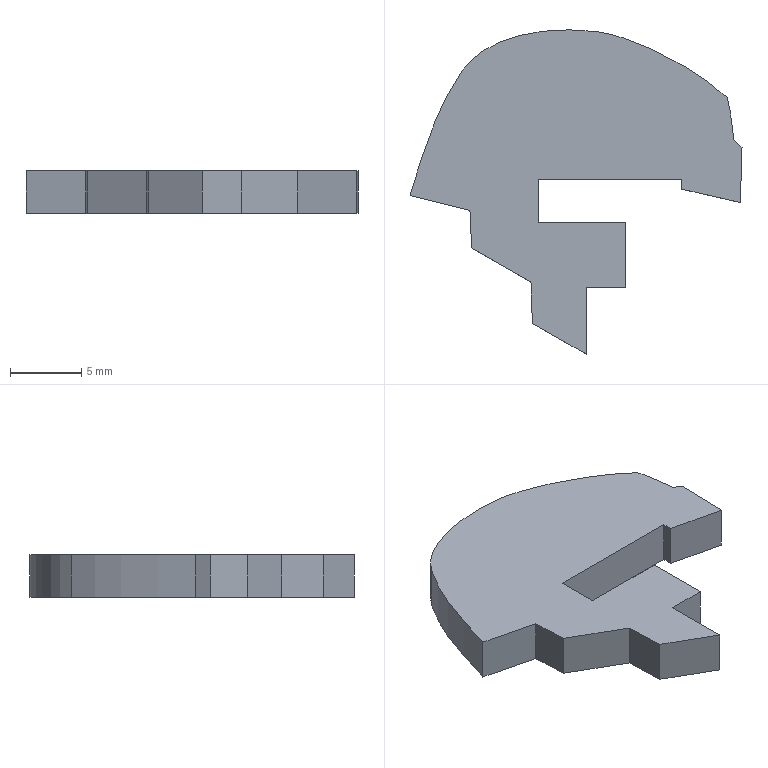Part | SolidWorks | features BaseBody 1 | 1 solid | 22 faces | box 23.312 x 22.774 x 3 mm | volume 818.077 mm3 | plane 18 | spline 4
STEP:
#1=CARTESIAN_POINT('',(21.406,16.89,-1.5));
#2=VERTEX_POINT('',#1);
#3=CARTESIAN_POINT('',(21.406,16.89,-1.5));
#4=VERTEX_POINT('',#3);
#5=CARTESIAN_POINT('',(21.406,16.89,-1.5));
#6=CARTESIAN_POINT('',(21.406,16.89,-1.5));
#7=CARTESIAN_POINT('',(21.406,16.89,-1.5));
#8=CARTESIAN_POINT('',(21.406,16.89,-1.5));
#9=B_SPLINE_CURVE_WITH_KNOTS('',3,(#5,#6,#7,#8),.UNSPECIFIED.,.F.,.F.,(4,4),(0.,0.000000108),.UNSPECIFIED.);
#10=EDGE_CURVE('',#2,#4,#9,.T.);
#11=ORIENTED_EDGE('',*,*,#10,.F.);
#12=CARTESIAN_POINT('',(25.034,25.614,-1.5));
#13=VERTEX_POINT('',#12);
#14=CARTESIAN_POINT('',(25.034,25.614,-1.5));
#15=CARTESIAN_POINT('',(23.262,23.049,-1.5));
#16=CARTESIAN_POINT('',(22.335,19.969,-1.5));
#17=CARTESIAN_POINT('',(21.406,16.89,-1.5));
#18=B_SPLINE_CURVE_WITH_KNOTS('',3,(#14,#15,#16,#17),.UNSPECIFIED.,.F.,.F.,(4,4),(0.000000108,0.03704),.UNSPECIFIED.);
#19=EDGE_CURVE('',#13,#2,#18,.T.);
#20=ORIENTED_EDGE('',*,*,#19,.F.);
#21=CARTESIAN_POINT('',(34.487,28.405,-1.5));
#22=VERTEX_POINT('',#21);
#23=CARTESIAN_POINT('',(34.487,28.405,-1.5));
#24=CARTESIAN_POINT('',(30.775,28.862,-1.5));
#25=CARTESIAN_POINT('',(26.734,28.074,-1.5));
#26=CARTESIAN_POINT('',(25.034,25.614,-1.5));
#27=B_SPLINE_CURVE_WITH_KNOTS('',3,(#23,#24,#25,#26),.UNSPECIFIED.,.F.,.F.,(4,4),(0.03704,0.07407),.UNSPECIFIED.);
#28=EDGE_CURVE('',#22,#13,#27,.T.);
#29=ORIENTED_EDGE('',*,*,#28,.F.);
#30=CARTESIAN_POINT('',(43.675,23.77,-1.5));
#31=VERTEX_POINT('',#30);
#32=CARTESIAN_POINT('',(43.675,23.77,-1.5));
#33=CARTESIAN_POINT('',(41.477,25.846,-1.5));
#34=CARTESIAN_POINT('',(37.107,28.083,-1.5));
#35=CARTESIAN_POINT('',(34.487,28.405,-1.5));
#36=B_SPLINE_CURVE_WITH_KNOTS('',3,(#32,#33,#34,#35),.UNSPECIFIED.,.F.,.F.,(4,4),(0.07407,0.1111),.UNSPECIFIED.);
#37=EDGE_CURVE('',#31,#22,#36,.T.);
#38=ORIENTED_EDGE('',*,*,#37,.F.);
#39=CARTESIAN_POINT('',(44.146,20.823,-1.5));
#40=VERTEX_POINT('',#39);
#41=CARTESIAN_POINT('',(44.146,20.823,-1.5));
#42=CARTESIAN_POINT('',(44.01,22.01,-1.5));
#43=CARTESIAN_POINT('',(43.871,23.199,-1.5));
#44=CARTESIAN_POINT('',(43.675,23.77,-1.5));
#45=B_SPLINE_CURVE_WITH_KNOTS('',3,(#41,#42,#43,#44),.UNSPECIFIED.,.F.,.F.,(4,4),(0.1111,0.1481),.UNSPECIFIED.);
#46=EDGE_CURVE('',#40,#31,#45,.T.);
#47=ORIENTED_EDGE('',*,*,#46,.F.);
#48=CARTESIAN_POINT('',(44.718,20.295,-1.5));
#49=VERTEX_POINT('',#48);
#50=CARTESIAN_POINT('',(44.718,20.295,-1.5));
#51=DIRECTION('',(-0.7346,0.6785,0.));
#52=VECTOR('',#51,1000.);
#53=LINE('',#50,#52);
#54=EDGE_CURVE('',#49,#40,#53,.T.);
#55=ORIENTED_EDGE('',*,*,#54,.F.);
#56=CARTESIAN_POINT('',(44.602,16.396,-1.5));
#57=VERTEX_POINT('',#56);
#58=CARTESIAN_POINT('',(44.602,16.396,-1.5));
#59=DIRECTION('',(0.02986,0.9996,0.));
#60=VECTOR('',#59,1000.);
#61=LINE('',#58,#60);
#62=EDGE_CURVE('',#57,#49,#61,.T.);
#63=ORIENTED_EDGE('',*,*,#62,.F.);
#64=CARTESIAN_POINT('',(40.499,17.339,-1.5));
#65=VERTEX_POINT('',#64);
#66=CARTESIAN_POINT('',(40.499,17.339,-1.5));
#67=DIRECTION('',(0.9746,-0.224,0.));
#68=VECTOR('',#67,1000.);
#69=LINE('',#66,#68);
#70=EDGE_CURVE('',#65,#57,#69,.T.);
#71=ORIENTED_EDGE('',*,*,#70,.F.);
#72=CARTESIAN_POINT('',(40.499,18.018,-1.5));
#73=VERTEX_POINT('',#72);
#74=CARTESIAN_POINT('',(40.499,18.018,-1.5));
#75=DIRECTION('',(0.,-1.,0.));
#76=VECTOR('',#75,1000.);
#77=LINE('',#74,#76);
#78=EDGE_CURVE('',#73,#65,#77,.T.);
#79=ORIENTED_EDGE('',*,*,#78,.F.);
#80=CARTESIAN_POINT('',(30.416,18.018,-1.5));
#81=VERTEX_POINT('',#80);
#82=CARTESIAN_POINT('',(30.416,18.018,-1.5));
#83=DIRECTION('',(1.,0.,0.));
#84=VECTOR('',#83,1000.);
#85=LINE('',#82,#84);
#86=EDGE_CURVE('',#81,#73,#85,.T.);
#87=ORIENTED_EDGE('',*,*,#86,.F.);
#88=CARTESIAN_POINT('',(30.416,15.018,-1.5));
#89=VERTEX_POINT('',#88);
#90=CARTESIAN_POINT('',(30.416,15.018,-1.5));
#91=DIRECTION('',(0.,1.,0.));
#92=VECTOR('',#91,1000.);
#93=LINE('',#90,#92);
#94=EDGE_CURVE('',#89,#81,#93,.T.);
#95=ORIENTED_EDGE('',*,*,#94,.F.);
#96=CARTESIAN_POINT('',(36.549,15.018,-1.5));
#97=VERTEX_POINT('',#96);
#98=CARTESIAN_POINT('',(36.549,15.018,-1.5));
#99=DIRECTION('',(-1.,0.,0.));
#100=VECTOR('',#99,1000.);
#101=LINE('',#98,#100);
#102=EDGE_CURVE('',#97,#89,#101,.T.);
#103=ORIENTED_EDGE('',*,*,#102,.F.);
#104=CARTESIAN_POINT('',(36.549,10.438,-1.5));
#105=VERTEX_POINT('',#104);
#106=CARTESIAN_POINT('',(36.549,10.438,-1.5));
#107=DIRECTION('',(0.,1.,0.));
#108=VECTOR('',#107,1000.);
#109=LINE('',#106,#108);
#110=EDGE_CURVE('',#105,#97,#109,.T.);
#111=ORIENTED_EDGE('',*,*,#110,.F.);
#112=CARTESIAN_POINT('',(33.779,10.438,-1.5));
#113=VERTEX_POINT('',#112);
#114=CARTESIAN_POINT('',(33.779,10.438,-1.5));
#115=DIRECTION('',(1.,0.,0.));
#116=VECTOR('',#115,1000.);
#117=LINE('',#114,#116);
#118=EDGE_CURVE('',#113,#105,#117,.T.);
#119=ORIENTED_EDGE('',*,*,#118,.F.);
#120=CARTESIAN_POINT('',(33.779,5.755,-1.5));
#121=VERTEX_POINT('',#120);
#122=CARTESIAN_POINT('',(33.779,5.755,-1.5));
#123=DIRECTION('',(0.,1.,0.));
#124=VECTOR('',#123,1000.);
#125=LINE('',#122,#124);
#126=EDGE_CURVE('',#121,#113,#125,.T.);
#127=ORIENTED_EDGE('',*,*,#126,.F.);
#128=CARTESIAN_POINT('',(29.997,7.91,-1.5));
#129=VERTEX_POINT('',#128);
#130=CARTESIAN_POINT('',(29.997,7.91,-1.5));
#131=DIRECTION('',(0.8688,-0.4952,0.));
#132=VECTOR('',#131,1000.);
#133=LINE('',#130,#132);
#134=EDGE_CURVE('',#129,#121,#133,.T.);
#135=ORIENTED_EDGE('',*,*,#134,.F.);
#136=CARTESIAN_POINT('',(29.9,10.832,-1.5));
#137=VERTEX_POINT('',#136);
#138=CARTESIAN_POINT('',(29.9,10.832,-1.5));
#139=DIRECTION('',(0.03337,-0.9994,0.));
#140=VECTOR('',#139,1000.);
#141=LINE('',#138,#140);
#142=EDGE_CURVE('',#137,#129,#141,.T.);
#143=ORIENTED_EDGE('',*,*,#142,.F.);
#144=CARTESIAN_POINT('',(25.734,13.212,-1.5));
#145=VERTEX_POINT('',#144);
#146=CARTESIAN_POINT('',(25.734,13.212,-1.5));
#147=DIRECTION('',(0.8682,-0.4962,0.));
#148=VECTOR('',#147,1000.);
#149=LINE('',#146,#148);
#150=EDGE_CURVE('',#145,#137,#149,.T.);
#151=ORIENTED_EDGE('',*,*,#150,.F.);
#152=CARTESIAN_POINT('',(25.615,15.852,-1.5));
#153=VERTEX_POINT('',#152);
#154=CARTESIAN_POINT('',(25.615,15.852,-1.5));
#155=DIRECTION('',(0.04529,-0.999,0.));
#156=VECTOR('',#155,1000.);
#157=LINE('',#154,#156);
#158=EDGE_CURVE('',#153,#145,#157,.T.);
#159=ORIENTED_EDGE('',*,*,#158,.F.);
#160=CARTESIAN_POINT('',(21.406,16.89,-1.5));
#161=DIRECTION('',(0.9709,-0.2396,0.));
#162=VECTOR('',#161,1000.);
#163=LINE('',#160,#162);
#164=EDGE_CURVE('',#4,#153,#163,.T.);
#165=ORIENTED_EDGE('',*,*,#164,.F.);
#166=EDGE_LOOP('',(#11,#20,#29,#38,#47,#55,#63,#71,#79,#87,#95,#103,#111,#119,#127,#135,#143,#151,#159,#165));
#167=FACE_OUTER_BOUND('',#166,.T.);
#168=CARTESIAN_POINT('',(22.904,21.445,-1.5));
#169=DIRECTION('',(0.,0.,-1.));
#170=DIRECTION('',(0.,-1.,0.));
#171=AXIS2_PLACEMENT_3D('',#168,#169,#170);
#172=PLANE('',#171);
#173=ADVANCED_FACE('',(#167),#172,.T.);
#174=CARTESIAN_POINT('',(21.406,16.89,1.5));
#175=VERTEX_POINT('',#174);
#176=CARTESIAN_POINT('',(21.406,16.89,1.5));
#177=VERTEX_POINT('',#176);
#178=CARTESIAN_POINT('',(21.406,16.89,1.5));
#179=CARTESIAN_POINT('',(21.406,16.89,1.5));
#180=CARTESIAN_POINT('',(21.406,16.89,1.5));
#181=CARTESIAN_POINT('',(21.406,16.89,1.5));
#182=B_SPLINE_CURVE_WITH_KNOTS('',3,(#178,#179,#180,#181),.UNSPECIFIED.,.F.,.F.,(4,4),(0.,0.000000108),.UNSPECIFIED.);
#183=EDGE_CURVE('',#175,#177,#182,.T.);
#184=ORIENTED_EDGE('',*,*,#183,.T.);
#185=CARTESIAN_POINT('',(25.615,15.852,1.5));
#186=VERTEX_POINT('',#185);
#187=CARTESIAN_POINT('',(21.406,16.89,1.5));
#188=DIRECTION('',(0.9709,-0.2396,0.));
#189=VECTOR('',#188,1000.);
#190=LINE('',#187,#189);
#191=EDGE_CURVE('',#177,#186,#190,.T.);
#192=ORIENTED_EDGE('',*,*,#191,.T.);
#193=CARTESIAN_POINT('',(25.734,13.212,1.5));
#194=VERTEX_POINT('',#193);
#195=CARTESIAN_POINT('',(25.615,15.852,1.5));
#196=DIRECTION('',(0.04529,-0.999,0.));
#197=VECTOR('',#196,1000.);
#198=LINE('',#195,#197);
#199=EDGE_CURVE('',#186,#194,#198,.T.);
#200=ORIENTED_EDGE('',*,*,#199,.T.);
#201=CARTESIAN_POINT('',(29.9,10.832,1.5));
#202=VERTEX_POINT('',#201);
#203=CARTESIAN_POINT('',(25.734,13.212,1.5));
#204=DIRECTION('',(0.8682,-0.4962,0.));
#205=VECTOR('',#204,1000.);
#206=LINE('',#203,#205);
#207=EDGE_CURVE('',#194,#202,#206,.T.);
#208=ORIENTED_EDGE('',*,*,#207,.T.);
#209=CARTESIAN_POINT('',(29.997,7.91,1.5));
#210=VERTEX_POINT('',#209);
#211=CARTESIAN_POINT('',(29.9,10.832,1.5));
#212=DIRECTION('',(0.03337,-0.9994,0.));
#213=VECTOR('',#212,1000.);
#214=LINE('',#211,#213);
#215=EDGE_CURVE('',#202,#210,#214,.T.);
#216=ORIENTED_EDGE('',*,*,#215,.T.);
#217=CARTESIAN_POINT('',(33.779,5.755,1.5));
#218=VERTEX_POINT('',#217);
#219=CARTESIAN_POINT('',(29.997,7.91,1.5));
#220=DIRECTION('',(0.8688,-0.4952,0.));
#221=VECTOR('',#220,1000.);
#222=LINE('',#219,#221);
#223=EDGE_CURVE('',#210,#218,#222,.T.);
#224=ORIENTED_EDGE('',*,*,#223,.T.);
#225=CARTESIAN_POINT('',(33.779,10.438,1.5));
#226=VERTEX_POINT('',#225);
#227=CARTESIAN_POINT('',(33.779,5.755,1.5));
#228=DIRECTION('',(0.,1.,0.));
#229=VECTOR('',#228,1000.);
#230=LINE('',#227,#229);
#231=EDGE_CURVE('',#218,#226,#230,.T.);
#232=ORIENTED_EDGE('',*,*,#231,.T.);
#233=CARTESIAN_POINT('',(36.549,10.438,1.5));
#234=VERTEX_POINT('',#233);
#235=CARTESIAN_POINT('',(33.779,10.438,1.5));
#236=DIRECTION('',(1.,0.,0.));
#237=VECTOR('',#236,1000.);
#238=LINE('',#235,#237);
#239=EDGE_CURVE('',#226,#234,#238,.T.);
#240=ORIENTED_EDGE('',*,*,#239,.T.);
#241=CARTESIAN_POINT('',(36.549,15.018,1.5));
#242=VERTEX_POINT('',#241);
#243=CARTESIAN_POINT('',(36.549,10.438,1.5));
#244=DIRECTION('',(0.,1.,0.));
#245=VECTOR('',#244,1000.);
#246=LINE('',#243,#245);
#247=EDGE_CURVE('',#234,#242,#246,.T.);
#248=ORIENTED_EDGE('',*,*,#247,.T.);
#249=CARTESIAN_POINT('',(30.416,15.018,1.5));
#250=VERTEX_POINT('',#249);
#251=CARTESIAN_POINT('',(36.549,15.018,1.5));
#252=DIRECTION('',(-1.,0.,0.));
#253=VECTOR('',#252,1000.);
#254=LINE('',#251,#253);
#255=EDGE_CURVE('',#242,#250,#254,.T.);
#256=ORIENTED_EDGE('',*,*,#255,.T.);
#257=CARTESIAN_POINT('',(30.416,18.018,1.5));
#258=VERTEX_POINT('',#257);
#259=CARTESIAN_POINT('',(30.416,15.018,1.5));
#260=DIRECTION('',(0.,1.,0.));
#261=VECTOR('',#260,1000.);
#262=LINE('',#259,#261);
#263=EDGE_CURVE('',#250,#258,#262,.T.);
#264=ORIENTED_EDGE('',*,*,#263,.T.);
#265=CARTESIAN_POINT('',(40.499,18.018,1.5));
#266=VERTEX_POINT('',#265);
#267=CARTESIAN_POINT('',(30.416,18.018,1.5));
#268=DIRECTION('',(1.,0.,0.));
#269=VECTOR('',#268,1000.);
#270=LINE('',#267,#269);
#271=EDGE_CURVE('',#258,#266,#270,.T.);
#272=ORIENTED_EDGE('',*,*,#271,.T.);
#273=CARTESIAN_POINT('',(40.499,17.339,1.5));
#274=VERTEX_POINT('',#273);
#275=CARTESIAN_POINT('',(40.499,18.018,1.5));
#276=DIRECTION('',(0.,-1.,0.));
#277=VECTOR('',#276,1000.);
#278=LINE('',#275,#277);
#279=EDGE_CURVE('',#266,#274,#278,.T.);
#280=ORIENTED_EDGE('',*,*,#279,.T.);
#281=CARTESIAN_POINT('',(44.602,16.396,1.5));
#282=VERTEX_POINT('',#281);
#283=CARTESIAN_POINT('',(40.499,17.339,1.5));
#284=DIRECTION('',(0.9746,-0.224,0.));
#285=VECTOR('',#284,1000.);
#286=LINE('',#283,#285);
#287=EDGE_CURVE('',#274,#282,#286,.T.);
#288=ORIENTED_EDGE('',*,*,#287,.T.);
#289=CARTESIAN_POINT('',(44.718,20.295,1.5));
#290=VERTEX_POINT('',#289);
#291=CARTESIAN_POINT('',(44.602,16.396,1.5));
#292=DIRECTION('',(0.02986,0.9996,0.));
#293=VECTOR('',#292,1000.);
#294=LINE('',#291,#293);
#295=EDGE_CURVE('',#282,#290,#294,.T.);
#296=ORIENTED_EDGE('',*,*,#295,.T.);
#297=CARTESIAN_POINT('',(44.146,20.823,1.5));
#298=VERTEX_POINT('',#297);
#299=CARTESIAN_POINT('',(44.718,20.295,1.5));
#300=DIRECTION('',(-0.7346,0.6785,0.));
#301=VECTOR('',#300,1000.);
#302=LINE('',#299,#301);
#303=EDGE_CURVE('',#290,#298,#302,.T.);
#304=ORIENTED_EDGE('',*,*,#303,.T.);
#305=CARTESIAN_POINT('',(43.675,23.77,1.5));
#306=VERTEX_POINT('',#305);
#307=CARTESIAN_POINT('',(44.146,20.823,1.5));
#308=CARTESIAN_POINT('',(44.01,22.01,1.5));
#309=CARTESIAN_POINT('',(43.871,23.199,1.5));
#310=CARTESIAN_POINT('',(43.675,23.77,1.5));
#311=B_SPLINE_CURVE_WITH_KNOTS('',3,(#307,#308,#309,#310),.UNSPECIFIED.,.F.,.F.,(4,4),(0.1111,0.1481),.UNSPECIFIED.);
#312=EDGE_CURVE('',#298,#306,#311,.T.);
#313=ORIENTED_EDGE('',*,*,#312,.T.);
#314=CARTESIAN_POINT('',(34.487,28.405,1.5));
#315=VERTEX_POINT('',#314);
#316=CARTESIAN_POINT('',(43.675,23.77,1.5));
#317=CARTESIAN_POINT('',(41.477,25.846,1.5));
#318=CARTESIAN_POINT('',(37.107,28.083,1.5));
#319=CARTESIAN_POINT('',(34.487,28.405,1.5));
#320=B_SPLINE_CURVE_WITH_KNOTS('',3,(#316,#317,#318,#319),.UNSPECIFIED.,.F.,.F.,(4,4),(0.07407,0.1111),.UNSPECIFIED.);
#321=EDGE_CURVE('',#306,#315,#320,.T.);
#322=ORIENTED_EDGE('',*,*,#321,.T.);
#323=CARTESIAN_POINT('',(25.034,25.614,1.5));
#324=VERTEX_POINT('',#323);
#325=CARTESIAN_POINT('',(34.487,28.405,1.5));
#326=CARTESIAN_POINT('',(30.775,28.862,1.5));
#327=CARTESIAN_POINT('',(26.734,28.074,1.5));
#328=CARTESIAN_POINT('',(25.034,25.614,1.5));
#329=B_SPLINE_CURVE_WITH_KNOTS('',3,(#325,#326,#327,#328),.UNSPECIFIED.,.F.,.F.,(4,4),(0.03704,0.07407),.UNSPECIFIED.);
#330=EDGE_CURVE('',#315,#324,#329,.T.);
#331=ORIENTED_EDGE('',*,*,#330,.T.);
#332=CARTESIAN_POINT('',(25.034,25.614,1.5));
#333=CARTESIAN_POINT('',(23.262,23.049,1.5));
#334=CARTESIAN_POINT('',(22.335,19.969,1.5));
#335=CARTESIAN_POINT('',(21.406,16.89,1.5));
#336=B_SPLINE_CURVE_WITH_KNOTS('',3,(#332,#333,#334,#335),.UNSPECIFIED.,.F.,.F.,(4,4),(0.000000108,0.03704),.UNSPECIFIED.);
#337=EDGE_CURVE('',#324,#175,#336,.T.);
#338=ORIENTED_EDGE('',*,*,#337,.T.);
#339=EDGE_LOOP('',(#184,#192,#200,#208,#216,#224,#232,#240,#248,#256,#264,#272,#280,#288,#296,#304,#313,#322,#331,#338));
#340=FACE_OUTER_BOUND('',#339,.T.);
#341=CARTESIAN_POINT('',(22.904,21.445,1.5));
#342=DIRECTION('',(0.,0.,-1.));
#343=DIRECTION('',(0.,-1.,0.));
#344=AXIS2_PLACEMENT_3D('',#341,#342,#343);
#345=PLANE('',#344);
#346=ADVANCED_FACE('',(#340),#345,.F.);
#347=ORIENTED_EDGE('',*,*,#19,.T.);
#348=CARTESIAN_POINT('',(21.406,16.89,1.5));
#349=DIRECTION('',(0.,0.,-1.));
#350=VECTOR('',#349,1000.);
#351=LINE('',#348,#350);
#352=EDGE_CURVE('',#175,#2,#351,.T.);
#353=ORIENTED_EDGE('',*,*,#352,.F.);
#354=ORIENTED_EDGE('',*,*,#337,.F.);
#355=CARTESIAN_POINT('',(25.034,25.614,1.5));
#356=DIRECTION('',(0.,0.,-1.));
#357=VECTOR('',#356,1000.);
#358=LINE('',#355,#357);
#359=EDGE_CURVE('',#324,#13,#358,.T.);
#360=ORIENTED_EDGE('',*,*,#359,.T.);
#361=EDGE_LOOP('',(#347,#353,#354,#360));
#362=FACE_OUTER_BOUND('',#361,.T.);
#363=CARTESIAN_POINT('',(25.034,25.614,1.5));
#364=CARTESIAN_POINT('',(25.034,25.614,-1.5));
#365=CARTESIAN_POINT('',(23.262,23.049,1.5));
#366=CARTESIAN_POINT('',(23.262,23.049,-1.5));
#367=CARTESIAN_POINT('',(22.335,19.969,1.5));
#368=CARTESIAN_POINT('',(22.335,19.969,-1.5));
#369=CARTESIAN_POINT('',(21.406,16.89,1.5));
#370=CARTESIAN_POINT('',(21.406,16.89,-1.5));
#371=B_SPLINE_SURFACE_WITH_KNOTS('',3,1,((#363,#364),(#365,#366),(#367,#368),(#369,#370)),.UNSPECIFIED.,.F.,.F.,.F.,(4,4),(2,2),(0.000000108,0.03704),(0.,1.),.UNSPECIFIED.);
#372=ADVANCED_FACE('',(#362),#371,.F.);
#373=ORIENTED_EDGE('',*,*,#28,.T.);
#374=ORIENTED_EDGE('',*,*,#359,.F.);
#375=ORIENTED_EDGE('',*,*,#330,.F.);
#376=CARTESIAN_POINT('',(34.487,28.405,1.5));
#377=DIRECTION('',(0.,0.,-1.));
#378=VECTOR('',#377,1000.);
#379=LINE('',#376,#378);
#380=EDGE_CURVE('',#315,#22,#379,.T.);
#381=ORIENTED_EDGE('',*,*,#380,.T.);
#382=EDGE_LOOP('',(#373,#374,#375,#381));
#383=FACE_OUTER_BOUND('',#382,.T.);
#384=CARTESIAN_POINT('',(34.487,28.405,1.5));
#385=CARTESIAN_POINT('',(34.487,28.405,-1.5));
#386=CARTESIAN_POINT('',(30.775,28.862,1.5));
#387=CARTESIAN_POINT('',(30.775,28.862,-1.5));
#388=CARTESIAN_POINT('',(26.734,28.074,1.5));
#389=CARTESIAN_POINT('',(26.734,28.074,-1.5));
#390=CARTESIAN_POINT('',(25.034,25.614,1.5));
#391=CARTESIAN_POINT('',(25.034,25.614,-1.5));
#392=B_SPLINE_SURFACE_WITH_KNOTS('',3,1,((#384,#385),(#386,#387),(#388,#389),(#390,#391)),.UNSPECIFIED.,.F.,.F.,.F.,(4,4),(2,2),(0.03704,0.07407),(0.,1.),.UNSPECIFIED.);
#393=ADVANCED_FACE('',(#383),#392,.F.);
#394=ORIENTED_EDGE('',*,*,#37,.T.);
#395=ORIENTED_EDGE('',*,*,#380,.F.);
#396=ORIENTED_EDGE('',*,*,#321,.F.);
#397=CARTESIAN_POINT('',(43.675,23.77,1.5));
#398=DIRECTION('',(0.,0.,-1.));
#399=VECTOR('',#398,1000.);
#400=LINE('',#397,#399);
#401=EDGE_CURVE('',#306,#31,#400,.T.);
#402=ORIENTED_EDGE('',*,*,#401,.T.);
#403=EDGE_LOOP('',(#394,#395,#396,#402));
#404=FACE_OUTER_BOUND('',#403,.T.);
#405=CARTESIAN_POINT('',(43.675,23.77,1.5));
#406=CARTESIAN_POINT('',(43.675,23.77,-1.5));
#407=CARTESIAN_POINT('',(41.477,25.846,1.5));
#408=CARTESIAN_POINT('',(41.477,25.846,-1.5));
#409=CARTESIAN_POINT('',(37.107,28.083,1.5));
#410=CARTESIAN_POINT('',(37.107,28.083,-1.5));
#411=CARTESIAN_POINT('',(34.487,28.405,1.5));
#412=CARTESIAN_POINT('',(34.487,28.405,-1.5));
#413=B_SPLINE_SURFACE_WITH_KNOTS('',3,1,((#405,#406),(#407,#408),(#409,#410),(#411,#412)),.UNSPECIFIED.,.F.,.F.,.F.,(4,4),(2,2),(0.07407,0.1111),(0.,1.),.UNSPECIFIED.);
#414=ADVANCED_FACE('',(#404),#413,.F.);
#415=ORIENTED_EDGE('',*,*,#46,.T.);
#416=ORIENTED_EDGE('',*,*,#401,.F.);
#417=ORIENTED_EDGE('',*,*,#312,.F.);
#418=CARTESIAN_POINT('',(44.146,20.823,1.5));
#419=DIRECTION('',(0.,0.,-1.));
#420=VECTOR('',#419,1000.);
#421=LINE('',#418,#420);
#422=EDGE_CURVE('',#298,#40,#421,.T.);
#423=ORIENTED_EDGE('',*,*,#422,.T.);
#424=EDGE_LOOP('',(#415,#416,#417,#423));
#425=FACE_OUTER_BOUND('',#424,.T.);
#426=CARTESIAN_POINT('',(44.146,20.823,1.5));
#427=CARTESIAN_POINT('',(44.146,20.823,-1.5));
#428=CARTESIAN_POINT('',(44.01,22.01,1.5));
#429=CARTESIAN_POINT('',(44.01,22.01,-1.5));
#430=CARTESIAN_POINT('',(43.871,23.199,1.5));
#431=CARTESIAN_POINT('',(43.871,23.199,-1.5));
#432=CARTESIAN_POINT('',(43.675,23.77,1.5));
#433=CARTESIAN_POINT('',(43.675,23.77,-1.5));
#434=B_SPLINE_SURFACE_WITH_KNOTS('',3,1,((#426,#427),(#428,#429),(#430,#431),(#432,#433)),.UNSPECIFIED.,.F.,.F.,.F.,(4,4),(2,2),(0.1111,0.1481),(0.,1.),.UNSPECIFIED.);
#435=ADVANCED_FACE('',(#425),#434,.F.);
#436=ORIENTED_EDGE('',*,*,#54,.T.);
#437=ORIENTED_EDGE('',*,*,#422,.F.);
#438=ORIENTED_EDGE('',*,*,#303,.F.);
#439=CARTESIAN_POINT('',(44.718,20.295,1.5));
#440=DIRECTION('',(0.,0.,-1.));
#441=VECTOR('',#440,1000.);
#442=LINE('',#439,#441);
#443=EDGE_CURVE('',#290,#49,#442,.T.);
#444=ORIENTED_EDGE('',*,*,#443,.T.);
#445=EDGE_LOOP('',(#436,#437,#438,#444));
#446=FACE_OUTER_BOUND('',#445,.T.);
#447=CARTESIAN_POINT('',(44.718,20.295,1.5));
#448=DIRECTION('',(-0.6785,-0.7346,0.));
#449=DIRECTION('',(-0.7346,0.6785,0.));
#450=AXIS2_PLACEMENT_3D('',#447,#448,#449);
#451=PLANE('',#450);
#452=ADVANCED_FACE('',(#446),#451,.F.);
#453=ORIENTED_EDGE('',*,*,#62,.T.);
#454=ORIENTED_EDGE('',*,*,#443,.F.);
#455=ORIENTED_EDGE('',*,*,#295,.F.);
#456=CARTESIAN_POINT('',(44.602,16.396,1.5));
#457=DIRECTION('',(0.,0.,-1.));
#458=VECTOR('',#457,1000.);
#459=LINE('',#456,#458);
#460=EDGE_CURVE('',#282,#57,#459,.T.);
#461=ORIENTED_EDGE('',*,*,#460,.T.);
#462=EDGE_LOOP('',(#453,#454,#455,#461));
#463=FACE_OUTER_BOUND('',#462,.T.);
#464=CARTESIAN_POINT('',(44.602,16.396,1.5));
#465=DIRECTION('',(-0.9996,0.02986,0.));
#466=DIRECTION('',(0.,0.,1.));
#467=AXIS2_PLACEMENT_3D('',#464,#465,#466);
#468=PLANE('',#467);
#469=ADVANCED_FACE('',(#463),#468,.F.);
#470=ORIENTED_EDGE('',*,*,#70,.T.);
#471=ORIENTED_EDGE('',*,*,#460,.F.);
#472=ORIENTED_EDGE('',*,*,#287,.F.);
#473=CARTESIAN_POINT('',(40.499,17.339,1.5));
#474=DIRECTION('',(0.,0.,-1.));
#475=VECTOR('',#474,1000.);
#476=LINE('',#473,#475);
#477=EDGE_CURVE('',#274,#65,#476,.T.);
#478=ORIENTED_EDGE('',*,*,#477,.T.);
#479=EDGE_LOOP('',(#470,#471,#472,#478));
#480=FACE_OUTER_BOUND('',#479,.T.);
#481=CARTESIAN_POINT('',(40.499,17.339,1.5));
#482=DIRECTION('',(0.224,0.9746,0.));
#483=DIRECTION('',(0.,0.,-1.));
#484=AXIS2_PLACEMENT_3D('',#481,#482,#483);
#485=PLANE('',#484);
#486=ADVANCED_FACE('',(#480),#485,.F.);
#487=ORIENTED_EDGE('',*,*,#78,.T.);
#488=ORIENTED_EDGE('',*,*,#477,.F.);
#489=ORIENTED_EDGE('',*,*,#279,.F.);
#490=CARTESIAN_POINT('',(40.499,18.018,1.5));
#491=DIRECTION('',(0.,0.,-1.));
#492=VECTOR('',#491,1000.);
#493=LINE('',#490,#492);
#494=EDGE_CURVE('',#266,#73,#493,.T.);
#495=ORIENTED_EDGE('',*,*,#494,.T.);
#496=EDGE_LOOP('',(#487,#488,#489,#495));
#497=FACE_OUTER_BOUND('',#496,.T.);
#498=CARTESIAN_POINT('',(40.499,18.018,1.5));
#499=DIRECTION('',(1.,0.,0.));
#500=DIRECTION('',(0.,1.,0.));
#501=AXIS2_PLACEMENT_3D('',#498,#499,#500);
#502=PLANE('',#501);
#503=ADVANCED_FACE('',(#497),#502,.F.);
#504=ORIENTED_EDGE('',*,*,#86,.T.);
#505=ORIENTED_EDGE('',*,*,#494,.F.);
#506=ORIENTED_EDGE('',*,*,#271,.F.);
#507=CARTESIAN_POINT('',(30.416,18.018,1.5));
#508=DIRECTION('',(0.,0.,-1.));
#509=VECTOR('',#508,1000.);
#510=LINE('',#507,#509);
#511=EDGE_CURVE('',#258,#81,#510,.T.);
#512=ORIENTED_EDGE('',*,*,#511,.T.);
#513=EDGE_LOOP('',(#504,#505,#506,#512));
#514=FACE_OUTER_BOUND('',#513,.T.);
#515=CARTESIAN_POINT('',(30.416,18.018,1.5));
#516=DIRECTION('',(0.,1.,0.));
#517=DIRECTION('',(1.,0.,0.));
#518=AXIS2_PLACEMENT_3D('',#515,#516,#517);
#519=PLANE('',#518);
#520=ADVANCED_FACE('',(#514),#519,.F.);
#521=ORIENTED_EDGE('',*,*,#94,.T.);
#522=ORIENTED_EDGE('',*,*,#511,.F.);
#523=ORIENTED_EDGE('',*,*,#263,.F.);
#524=CARTESIAN_POINT('',(30.416,15.018,1.5));
#525=DIRECTION('',(0.,0.,-1.));
#526=VECTOR('',#525,1000.);
#527=LINE('',#524,#526);
#528=EDGE_CURVE('',#250,#89,#527,.T.);
#529=ORIENTED_EDGE('',*,*,#528,.T.);
#530=EDGE_LOOP('',(#521,#522,#523,#529));
#531=FACE_OUTER_BOUND('',#530,.T.);
#532=CARTESIAN_POINT('',(30.416,15.018,1.5));
#533=DIRECTION('',(-1.,0.,0.));
#534=DIRECTION('',(0.,0.,1.));
#535=AXIS2_PLACEMENT_3D('',#532,#533,#534);
#536=PLANE('',#535);
#537=ADVANCED_FACE('',(#531),#536,.F.);
#538=ORIENTED_EDGE('',*,*,#102,.T.);
#539=ORIENTED_EDGE('',*,*,#528,.F.);
#540=ORIENTED_EDGE('',*,*,#255,.F.);
#541=CARTESIAN_POINT('',(36.549,15.018,1.5));
#542=DIRECTION('',(0.,0.,-1.));
#543=VECTOR('',#542,1000.);
#544=LINE('',#541,#543);
#545=EDGE_CURVE('',#242,#97,#544,.T.);
#546=ORIENTED_EDGE('',*,*,#545,.T.);
#547=EDGE_LOOP('',(#538,#539,#540,#546));
#548=FACE_OUTER_BOUND('',#547,.T.);
#549=CARTESIAN_POINT('',(36.549,15.018,1.5));
#550=DIRECTION('',(0.,-1.,0.));
#551=DIRECTION('',(0.,0.,-1.));
#552=AXIS2_PLACEMENT_3D('',#549,#550,#551);
#553=PLANE('',#552);
#554=ADVANCED_FACE('',(#548),#553,.F.);
#555=ORIENTED_EDGE('',*,*,#110,.T.);
#556=ORIENTED_EDGE('',*,*,#545,.F.);
#557=ORIENTED_EDGE('',*,*,#247,.F.);
#558=CARTESIAN_POINT('',(36.549,10.438,1.5));
#559=DIRECTION('',(0.,0.,-1.));
#560=VECTOR('',#559,1000.);
#561=LINE('',#558,#560);
#562=EDGE_CURVE('',#234,#105,#561,.T.);
#563=ORIENTED_EDGE('',*,*,#562,.T.);
#564=EDGE_LOOP('',(#555,#556,#557,#563));
#565=FACE_OUTER_BOUND('',#564,.T.);
#566=CARTESIAN_POINT('',(36.549,10.438,1.5));
#567=DIRECTION('',(-1.,0.,0.));
#568=DIRECTION('',(0.,0.,1.));
#569=AXIS2_PLACEMENT_3D('',#566,#567,#568);
#570=PLANE('',#569);
#571=ADVANCED_FACE('',(#565),#570,.F.);
#572=ORIENTED_EDGE('',*,*,#118,.T.);
#573=ORIENTED_EDGE('',*,*,#562,.F.);
#574=ORIENTED_EDGE('',*,*,#239,.F.);
#575=CARTESIAN_POINT('',(33.779,10.438,1.5));
#576=DIRECTION('',(0.,0.,-1.));
#577=VECTOR('',#576,1000.);
#578=LINE('',#575,#577);
#579=EDGE_CURVE('',#226,#113,#578,.T.);
#580=ORIENTED_EDGE('',*,*,#579,.T.);
#581=EDGE_LOOP('',(#572,#573,#574,#580));
#582=FACE_OUTER_BOUND('',#581,.T.);
#583=CARTESIAN_POINT('',(33.779,10.438,1.5));
#584=DIRECTION('',(0.,1.,0.));
#585=DIRECTION('',(1.,0.,0.));
#586=AXIS2_PLACEMENT_3D('',#583,#584,#585);
#587=PLANE('',#586);
#588=ADVANCED_FACE('',(#582),#587,.F.);
#589=ORIENTED_EDGE('',*,*,#126,.T.);
#590=ORIENTED_EDGE('',*,*,#579,.F.);
#591=ORIENTED_EDGE('',*,*,#231,.F.);
#592=CARTESIAN_POINT('',(33.779,5.755,1.5));
#593=DIRECTION('',(0.,0.,-1.));
#594=VECTOR('',#593,1000.);
#595=LINE('',#592,#594);
#596=EDGE_CURVE('',#218,#121,#595,.T.);
#597=ORIENTED_EDGE('',*,*,#596,.T.);
#598=EDGE_LOOP('',(#589,#590,#591,#597));
#599=FACE_OUTER_BOUND('',#598,.T.);
#600=CARTESIAN_POINT('',(33.779,5.755,1.5));
#601=DIRECTION('',(-1.,0.,0.));
#602=DIRECTION('',(0.,0.,1.));
#603=AXIS2_PLACEMENT_3D('',#600,#601,#602);
#604=PLANE('',#603);
#605=ADVANCED_FACE('',(#599),#604,.F.);
#606=ORIENTED_EDGE('',*,*,#134,.T.);
#607=ORIENTED_EDGE('',*,*,#596,.F.);
#608=ORIENTED_EDGE('',*,*,#223,.F.);
#609=CARTESIAN_POINT('',(29.997,7.91,1.5));
#610=DIRECTION('',(0.,0.,-1.));
#611=VECTOR('',#610,1000.);
#612=LINE('',#609,#611);
#613=EDGE_CURVE('',#210,#129,#612,.T.);
#614=ORIENTED_EDGE('',*,*,#613,.T.);
#615=EDGE_LOOP('',(#606,#607,#608,#614));
#616=FACE_OUTER_BOUND('',#615,.T.);
#617=CARTESIAN_POINT('',(29.997,7.91,1.5));
#618=DIRECTION('',(0.4952,0.8688,0.));
#619=DIRECTION('',(0.,0.,-1.));
#620=AXIS2_PLACEMENT_3D('',#617,#618,#619);
#621=PLANE('',#620);
#622=ADVANCED_FACE('',(#616),#621,.F.);
#623=ORIENTED_EDGE('',*,*,#142,.T.);
#624=ORIENTED_EDGE('',*,*,#613,.F.);
#625=ORIENTED_EDGE('',*,*,#215,.F.);
#626=CARTESIAN_POINT('',(29.9,10.832,1.5));
#627=DIRECTION('',(0.,0.,-1.));
#628=VECTOR('',#627,1000.);
#629=LINE('',#626,#628);
#630=EDGE_CURVE('',#202,#137,#629,.T.);
#631=ORIENTED_EDGE('',*,*,#630,.T.);
#632=EDGE_LOOP('',(#623,#624,#625,#631));
#633=FACE_OUTER_BOUND('',#632,.T.);
#634=CARTESIAN_POINT('',(29.9,10.832,1.5));
#635=DIRECTION('',(0.9994,0.03337,0.));
#636=DIRECTION('',(0.,0.,-1.));
#637=AXIS2_PLACEMENT_3D('',#634,#635,#636);
#638=PLANE('',#637);
#639=ADVANCED_FACE('',(#633),#638,.F.);
#640=ORIENTED_EDGE('',*,*,#150,.T.);
#641=ORIENTED_EDGE('',*,*,#630,.F.);
#642=ORIENTED_EDGE('',*,*,#207,.F.);
#643=CARTESIAN_POINT('',(25.734,13.212,1.5));
#644=DIRECTION('',(0.,0.,-1.));
#645=VECTOR('',#644,1000.);
#646=LINE('',#643,#645);
#647=EDGE_CURVE('',#194,#145,#646,.T.);
#648=ORIENTED_EDGE('',*,*,#647,.T.);
#649=EDGE_LOOP('',(#640,#641,#642,#648));
#650=FACE_OUTER_BOUND('',#649,.T.);
#651=CARTESIAN_POINT('',(25.734,13.212,1.5));
#652=DIRECTION('',(0.4962,0.8682,0.));
#653=DIRECTION('',(0.,0.,-1.));
#654=AXIS2_PLACEMENT_3D('',#651,#652,#653);
#655=PLANE('',#654);
#656=ADVANCED_FACE('',(#650),#655,.F.);
#657=ORIENTED_EDGE('',*,*,#158,.T.);
#658=ORIENTED_EDGE('',*,*,#647,.F.);
#659=ORIENTED_EDGE('',*,*,#199,.F.);
#660=CARTESIAN_POINT('',(25.615,15.852,1.5));
#661=DIRECTION('',(0.,0.,-1.));
#662=VECTOR('',#661,1000.);
#663=LINE('',#660,#662);
#664=EDGE_CURVE('',#186,#153,#663,.T.);
#665=ORIENTED_EDGE('',*,*,#664,.T.);
#666=EDGE_LOOP('',(#657,#658,#659,#665));
#667=FACE_OUTER_BOUND('',#666,.T.);
#668=CARTESIAN_POINT('',(25.615,15.852,1.5));
#669=DIRECTION('',(0.999,0.04529,0.));
#670=DIRECTION('',(0.,0.,-1.));
#671=AXIS2_PLACEMENT_3D('',#668,#669,#670);
#672=PLANE('',#671);
#673=ADVANCED_FACE('',(#667),#672,.F.);
#674=ORIENTED_EDGE('',*,*,#164,.T.);
#675=ORIENTED_EDGE('',*,*,#664,.F.);
#676=ORIENTED_EDGE('',*,*,#191,.F.);
#677=CARTESIAN_POINT('',(21.406,16.89,1.5));
#678=DIRECTION('',(0.,0.,-1.));
#679=VECTOR('',#678,1000.);
#680=LINE('',#677,#679);
#681=EDGE_CURVE('',#177,#4,#680,.T.);
#682=ORIENTED_EDGE('',*,*,#681,.T.);
#683=EDGE_LOOP('',(#674,#675,#676,#682));
#684=FACE_OUTER_BOUND('',#683,.T.);
#685=CARTESIAN_POINT('',(21.406,16.89,1.5));
#686=DIRECTION('',(0.2396,0.9709,0.));
#687=DIRECTION('',(0.,0.,-1.));
#688=AXIS2_PLACEMENT_3D('',#685,#686,#687);
#689=PLANE('',#688);
#690=ADVANCED_FACE('',(#684),#689,.F.);
#691=ORIENTED_EDGE('',*,*,#10,.T.);
#692=ORIENTED_EDGE('',*,*,#681,.F.);
#693=ORIENTED_EDGE('',*,*,#183,.F.);
#694=ORIENTED_EDGE('',*,*,#352,.T.);
#695=EDGE_LOOP('',(#691,#692,#693,#694));
#696=FACE_OUTER_BOUND('',#695,.T.);
#697=CARTESIAN_POINT('',(21.406,16.89,1.5));
#698=DIRECTION('',(0.9574,-0.2888,0.));
#699=DIRECTION('',(0.,0.,-1.));
#700=AXIS2_PLACEMENT_3D('',#697,#698,#699);
#701=PLANE('',#700);
#702=ADVANCED_FACE('',(#696),#701,.F.);
#703=CLOSED_SHELL('',(#173,#346,#372,#393,#414,#435,#452,#469,#486,#503,#520,#537,#554,#571,#588,#605,#622,#639,#656,#673,#690,#702));
#704=MANIFOLD_SOLID_BREP('',#703);
#705=CARTESIAN_POINT('',(0.,0.,0.));
#706=DIRECTION('',(0.,0.,1.));
#707=DIRECTION('',(1.,0.,0.));
#708=AXIS2_PLACEMENT_3D('',#705,#706,#707);
#709=(LENGTH_UNIT()NAMED_UNIT(*)SI_UNIT(.MILLI.,.METRE.));
#710=UNCERTAINTY_MEASURE_WITH_UNIT(LENGTH_MEASURE(0.00001),#709,'','');
#711=(NAMED_UNIT(*)PLANE_ANGLE_UNIT()SI_UNIT($,.RADIAN.));
#712=(NAMED_UNIT(*)SI_UNIT($,.STERADIAN.)SOLID_ANGLE_UNIT());
#713=(GEOMETRIC_REPRESENTATION_CONTEXT(3)GLOBAL_UNCERTAINTY_ASSIGNED_CONTEXT((#710))GLOBAL_UNIT_ASSIGNED_CONTEXT((#709,#711,#712))REPRESENTATION_CONTEXT('',''));
#714=ADVANCED_BREP_SHAPE_REPRESENTATION('',(#704,#708),#713);